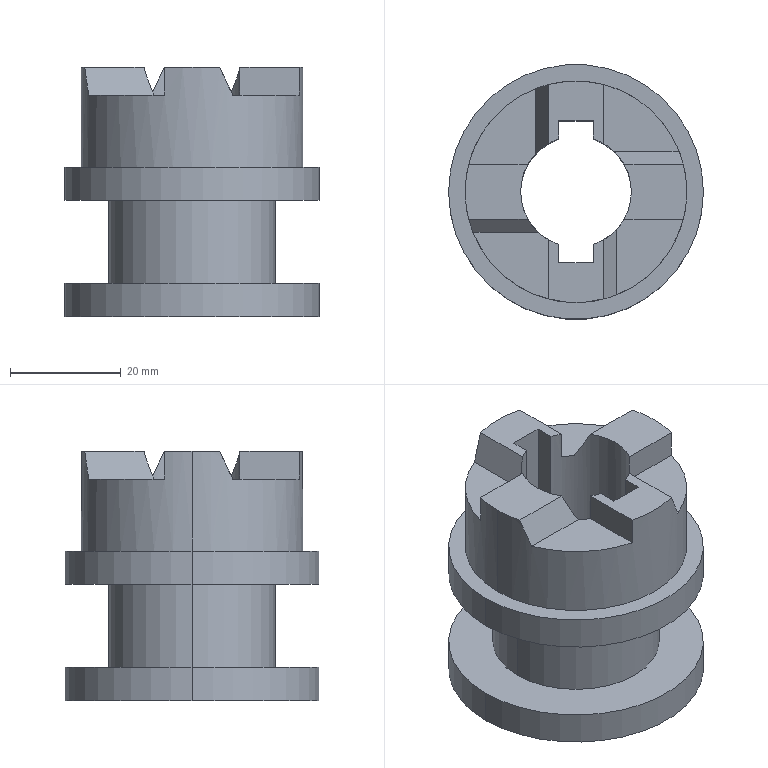Part | NX | features BREP 1, DATUM_CSYS 1, EXTRACT_DATUM_PLANE 1, SKETCH 1 | 1 solid | 37 faces | box 46 x 46 x 45 mm | volume 34964 mm3 | plane 26 | cylinder 11 | commonest cylinder face diameters 46 x4 20 x3 30 x2 40 x2
STEP:
#1=CARTESIAN_POINT('',(3.1,-12.8,45.));
#2=VERTEX_POINT('',#1);
#3=CARTESIAN_POINT('',(3.1,-12.8,0.));
#4=VERTEX_POINT('',#3);
#5=CARTESIAN_POINT('',(3.1,-12.8,45.));
#6=DIRECTION('',(0.,0.,-1.));
#7=VECTOR('',#6,1000.);
#8=LINE('',#5,#7);
#9=EDGE_CURVE('',#2,#4,#8,.T.);
#10=ORIENTED_EDGE('',*,*,#9,.T.);
#11=CARTESIAN_POINT('',(-3.1,-12.8,0.));
#12=VERTEX_POINT('',#11);
#13=CARTESIAN_POINT('',(3.1,-12.8,0.));
#14=DIRECTION('',(-1.,0.,0.));
#15=VECTOR('',#14,1000.);
#16=LINE('',#13,#15);
#17=EDGE_CURVE('',#4,#12,#16,.T.);
#18=ORIENTED_EDGE('',*,*,#17,.T.);
#19=CARTESIAN_POINT('',(-3.1,-12.8,45.));
#20=VERTEX_POINT('',#19);
#21=CARTESIAN_POINT('',(-3.1,-12.8,45.));
#22=DIRECTION('',(0.,0.,-1.));
#23=VECTOR('',#22,1000.);
#24=LINE('',#21,#23);
#25=EDGE_CURVE('',#20,#12,#24,.T.);
#26=ORIENTED_EDGE('',*,*,#25,.F.);
#27=CARTESIAN_POINT('',(3.1,-12.8,45.));
#28=DIRECTION('',(-1.,0.,0.));
#29=VECTOR('',#28,1000.);
#30=LINE('',#27,#29);
#31=EDGE_CURVE('',#2,#20,#30,.T.);
#32=ORIENTED_EDGE('',*,*,#31,.F.);
#33=EDGE_LOOP('',(#10,#18,#26,#32));
#34=FACE_BOUND('',#33,.T.);
#35=CARTESIAN_POINT('',(-3.1,-12.8,0.));
#36=DIRECTION('',(0.,-1.,0.));
#37=DIRECTION('',(0.,0.,1.));
#38=AXIS2_PLACEMENT_3D('',#35,#36,#37);
#39=PLANE('',#38);
#40=ADVANCED_FACE('',(#34),#39,.F.);
#41=CARTESIAN_POINT('',(-3.1,-9.507,45.));
#42=VERTEX_POINT('',#41);
#43=CARTESIAN_POINT('',(-3.1,-12.8,45.));
#44=DIRECTION('',(0.,1.,0.));
#45=VECTOR('',#44,1000.);
#46=LINE('',#43,#45);
#47=EDGE_CURVE('',#20,#42,#46,.T.);
#48=ORIENTED_EDGE('',*,*,#47,.T.);
#49=CARTESIAN_POINT('',(-5.,-8.66,45.));
#50=VERTEX_POINT('',#49);
#51=CARTESIAN_POINT('',(0.,0.,45.));
#52=DIRECTION('',(0.,0.,-1.));
#53=DIRECTION('',(-0.31,-0.9507,0.));
#54=AXIS2_PLACEMENT_3D('',#51,#52,#53);
#55=CIRCLE('',#54,10.);
#56=EDGE_CURVE('',#42,#50,#55,.T.);
#57=ORIENTED_EDGE('',*,*,#56,.T.);
#58=CARTESIAN_POINT('',(-5.,-19.365,45.));
#59=VERTEX_POINT('',#58);
#60=CARTESIAN_POINT('',(-5.,-8.66,45.));
#61=DIRECTION('',(0.,-1.,0.));
#62=VECTOR('',#61,1000.);
#63=LINE('',#60,#62);
#64=EDGE_CURVE('',#50,#59,#63,.T.);
#65=ORIENTED_EDGE('',*,*,#64,.T.);
#66=CARTESIAN_POINT('',(5.,-19.365,45.));
#67=VERTEX_POINT('',#66);
#68=CARTESIAN_POINT('',(0.,0.,45.));
#69=DIRECTION('',(0.,0.,1.));
#70=DIRECTION('',(-0.25,-0.9682,0.));
#71=AXIS2_PLACEMENT_3D('',#68,#69,#70);
#72=CIRCLE('',#71,20.);
#73=EDGE_CURVE('',#59,#67,#72,.T.);
#74=ORIENTED_EDGE('',*,*,#73,.T.);
#75=CARTESIAN_POINT('',(5.,-8.66,45.));
#76=VERTEX_POINT('',#75);
#77=CARTESIAN_POINT('',(5.,-8.66,45.));
#78=DIRECTION('',(0.,-1.,0.));
#79=VECTOR('',#78,1000.);
#80=LINE('',#77,#79);
#81=EDGE_CURVE('',#76,#67,#80,.T.);
#82=ORIENTED_EDGE('',*,*,#81,.F.);
#83=CARTESIAN_POINT('',(3.1,-9.507,45.));
#84=VERTEX_POINT('',#83);
#85=CARTESIAN_POINT('',(0.,0.,45.));
#86=DIRECTION('',(0.,0.,-1.));
#87=DIRECTION('',(0.5,-0.866,0.));
#88=AXIS2_PLACEMENT_3D('',#85,#86,#87);
#89=CIRCLE('',#88,10.);
#90=EDGE_CURVE('',#76,#84,#89,.T.);
#91=ORIENTED_EDGE('',*,*,#90,.T.);
#92=CARTESIAN_POINT('',(3.1,-9.507,45.));
#93=DIRECTION('',(0.,-1.,0.));
#94=VECTOR('',#93,1000.);
#95=LINE('',#92,#94);
#96=EDGE_CURVE('',#84,#2,#95,.T.);
#97=ORIENTED_EDGE('',*,*,#96,.T.);
#98=ORIENTED_EDGE('',*,*,#31,.T.);
#99=EDGE_LOOP('',(#48,#57,#65,#74,#82,#91,#97,#98));
#100=FACE_BOUND('',#99,.T.);
#101=CARTESIAN_POINT('',(-5.,28.,45.));
#102=DIRECTION('',(0.,0.,-1.));
#103=DIRECTION('',(1.,0.,0.));
#104=AXIS2_PLACEMENT_3D('',#101,#102,#103);
#105=PLANE('',#104);
#106=ADVANCED_FACE('',(#100),#105,.F.);
#107=CARTESIAN_POINT('',(3.1,-9.507,0.));
#108=VERTEX_POINT('',#107);
#109=CARTESIAN_POINT('',(3.1,-9.507,0.));
#110=DIRECTION('',(0.,-1.,0.));
#111=VECTOR('',#110,1000.);
#112=LINE('',#109,#111);
#113=EDGE_CURVE('',#108,#4,#112,.T.);
#114=ORIENTED_EDGE('',*,*,#113,.T.);
#115=ORIENTED_EDGE('',*,*,#9,.F.);
#116=ORIENTED_EDGE('',*,*,#96,.F.);
#117=CARTESIAN_POINT('',(3.1,-9.507,0.));
#118=DIRECTION('',(0.,0.,1.));
#119=VECTOR('',#118,1000.);
#120=LINE('',#117,#119);
#121=EDGE_CURVE('',#108,#84,#120,.T.);
#122=ORIENTED_EDGE('',*,*,#121,.F.);
#123=EDGE_LOOP('',(#114,#115,#116,#122));
#124=FACE_BOUND('',#123,.T.);
#125=CARTESIAN_POINT('',(3.1,-12.8,0.));
#126=DIRECTION('',(1.,0.,0.));
#127=DIRECTION('',(0.,-1.,0.));
#128=AXIS2_PLACEMENT_3D('',#125,#126,#127);
#129=PLANE('',#128);
#130=ADVANCED_FACE('',(#124),#129,.F.);
#131=ORIENTED_EDGE('',*,*,#90,.F.);
#132=CARTESIAN_POINT('',(7.332,-6.801,40.));
#133=VERTEX_POINT('',#132);
#134=CARTESIAN_POINT('',(0.,0.,55.723));
#135=DIRECTION('',(-0.9063,0.,-0.4226));
#136=DIRECTION('',(0.4226,0.,-0.9063));
#137=AXIS2_PLACEMENT_3D('',#134,#135,#136);
#138=ELLIPSE('',#137,23.662,10.);
#139=EDGE_CURVE('',#133,#76,#138,.T.);
#140=ORIENTED_EDGE('',*,*,#139,.F.);
#141=CARTESIAN_POINT('',(8.66,-5.,40.));
#142=VERTEX_POINT('',#141);
#143=CARTESIAN_POINT('',(0.,0.,40.));
#144=DIRECTION('',(0.,0.,-1.));
#145=DIRECTION('',(0.866,-0.5,0.));
#146=AXIS2_PLACEMENT_3D('',#143,#144,#145);
#147=CIRCLE('',#146,10.);
#148=EDGE_CURVE('',#142,#133,#147,.T.);
#149=ORIENTED_EDGE('',*,*,#148,.F.);
#150=CARTESIAN_POINT('',(8.66,-5.,45.));
#151=VERTEX_POINT('',#150);
#152=CARTESIAN_POINT('',(8.66,-5.,40.));
#153=DIRECTION('',(0.000000002,0.,1.));
#154=VECTOR('',#153,1000.);
#155=LINE('',#152,#154);
#156=EDGE_CURVE('',#142,#151,#155,.T.);
#157=ORIENTED_EDGE('',*,*,#156,.T.);
#158=CARTESIAN_POINT('',(10.,0.,45.));
#159=VERTEX_POINT('',#158);
#160=CARTESIAN_POINT('',(0.,0.,45.));
#161=DIRECTION('',(0.,0.,-1.));
#162=DIRECTION('',(1.,0.,0.));
#163=AXIS2_PLACEMENT_3D('',#160,#161,#162);
#164=CIRCLE('',#163,10.);
#165=EDGE_CURVE('',#159,#151,#164,.T.);
#166=ORIENTED_EDGE('',*,*,#165,.F.);
#167=CARTESIAN_POINT('',(8.66,5.,45.));
#168=VERTEX_POINT('',#167);
#169=CARTESIAN_POINT('',(0.,0.,45.));
#170=DIRECTION('',(0.,0.,-1.));
#171=DIRECTION('',(0.866,0.5,0.));
#172=AXIS2_PLACEMENT_3D('',#169,#170,#171);
#173=CIRCLE('',#172,10.);
#174=EDGE_CURVE('',#168,#159,#173,.T.);
#175=ORIENTED_EDGE('',*,*,#174,.F.);
#176=CARTESIAN_POINT('',(6.801,7.332,40.));
#177=VERTEX_POINT('',#176);
#178=CARTESIAN_POINT('',(0.,0.,55.723));
#179=DIRECTION('',(0.,-0.9063,-0.4226));
#180=DIRECTION('',(0.,0.4226,-0.9063));
#181=AXIS2_PLACEMENT_3D('',#178,#179,#180);
#182=ELLIPSE('',#181,23.662,10.);
#183=EDGE_CURVE('',#177,#168,#182,.T.);
#184=ORIENTED_EDGE('',*,*,#183,.F.);
#185=CARTESIAN_POINT('',(5.,8.66,40.));
#186=VERTEX_POINT('',#185);
#187=CARTESIAN_POINT('',(0.,0.,40.));
#188=DIRECTION('',(0.,0.,-1.));
#189=DIRECTION('',(0.5,0.866,0.));
#190=AXIS2_PLACEMENT_3D('',#187,#188,#189);
#191=CIRCLE('',#190,10.);
#192=EDGE_CURVE('',#186,#177,#191,.T.);
#193=ORIENTED_EDGE('',*,*,#192,.F.);
#194=CARTESIAN_POINT('',(5.,8.66,45.));
#195=VERTEX_POINT('',#194);
#196=CARTESIAN_POINT('',(5.,8.66,40.));
#197=DIRECTION('',(0.,0.000000001,1.));
#198=VECTOR('',#197,1000.);
#199=LINE('',#196,#198);
#200=EDGE_CURVE('',#186,#195,#199,.T.);
#201=ORIENTED_EDGE('',*,*,#200,.T.);
#202=CARTESIAN_POINT('',(3.1,9.507,45.));
#203=VERTEX_POINT('',#202);
#204=CARTESIAN_POINT('',(0.,0.,45.));
#205=DIRECTION('',(0.,0.,-1.));
#206=DIRECTION('',(0.31,0.9507,0.));
#207=AXIS2_PLACEMENT_3D('',#204,#205,#206);
#208=CIRCLE('',#207,10.);
#209=EDGE_CURVE('',#203,#195,#208,.T.);
#210=ORIENTED_EDGE('',*,*,#209,.F.);
#211=CARTESIAN_POINT('',(3.1,9.507,0.));
#212=VERTEX_POINT('',#211);
#213=CARTESIAN_POINT('',(3.1,9.507,45.));
#214=DIRECTION('',(0.,0.,-1.));
#215=VECTOR('',#214,1000.);
#216=LINE('',#213,#215);
#217=EDGE_CURVE('',#203,#212,#216,.T.);
#218=ORIENTED_EDGE('',*,*,#217,.T.);
#219=CARTESIAN_POINT('',(0.,0.,0.));
#220=DIRECTION('',(0.,0.,1.));
#221=DIRECTION('',(0.31,-0.9507,0.));
#222=AXIS2_PLACEMENT_3D('',#219,#220,#221);
#223=CIRCLE('',#222,10.);
#224=EDGE_CURVE('',#108,#212,#223,.T.);
#225=ORIENTED_EDGE('',*,*,#224,.F.);
#226=ORIENTED_EDGE('',*,*,#121,.T.);
#227=EDGE_LOOP('',(#131,#140,#149,#157,#166,#175,#184,#193,#201,#210,#218,#225,#226));
#228=FACE_BOUND('',#227,.T.);
#229=CARTESIAN_POINT('',(0.,0.,40.));
#230=DIRECTION('',(0.,0.,-1.));
#231=DIRECTION('',(1.,0.,0.));
#232=AXIS2_PLACEMENT_3D('',#229,#230,#231);
#233=CYLINDRICAL_SURFACE('',#232,10.);
#234=ADVANCED_FACE('',(#228),#233,.F.);
#235=CARTESIAN_POINT('',(23.,0.,0.));
#236=VERTEX_POINT('',#235);
#237=CARTESIAN_POINT('',(-23.,0.,0.));
#238=VERTEX_POINT('',#237);
#239=CARTESIAN_POINT('',(0.,0.,0.));
#240=DIRECTION('',(0.,0.,-1.));
#241=DIRECTION('',(1.,0.,0.));
#242=AXIS2_PLACEMENT_3D('',#239,#240,#241);
#243=CIRCLE('',#242,23.);
#244=EDGE_CURVE('',#236,#238,#243,.T.);
#245=ORIENTED_EDGE('',*,*,#244,.T.);
#246=CARTESIAN_POINT('',(0.,0.,0.));
#247=DIRECTION('',(0.,0.,-1.));
#248=DIRECTION('',(-1.,0.,0.));
#249=AXIS2_PLACEMENT_3D('',#246,#247,#248);
#250=CIRCLE('',#249,23.);
#251=EDGE_CURVE('',#238,#236,#250,.T.);
#252=ORIENTED_EDGE('',*,*,#251,.T.);
#253=EDGE_LOOP('',(#245,#252));
#254=FACE_BOUND('',#253,.T.);
#255=CARTESIAN_POINT('',(-10.,0.,0.));
#256=VERTEX_POINT('',#255);
#257=CARTESIAN_POINT('',(-3.1,-9.507,0.));
#258=VERTEX_POINT('',#257);
#259=CARTESIAN_POINT('',(0.,0.,0.));
#260=DIRECTION('',(0.,0.,1.));
#261=DIRECTION('',(-1.,0.,0.));
#262=AXIS2_PLACEMENT_3D('',#259,#260,#261);
#263=CIRCLE('',#262,10.);
#264=EDGE_CURVE('',#256,#258,#263,.T.);
#265=ORIENTED_EDGE('',*,*,#264,.T.);
#266=CARTESIAN_POINT('',(-3.1,-12.8,0.));
#267=DIRECTION('',(0.,1.,0.));
#268=VECTOR('',#267,1000.);
#269=LINE('',#266,#268);
#270=EDGE_CURVE('',#12,#258,#269,.T.);
#271=ORIENTED_EDGE('',*,*,#270,.F.);
#272=ORIENTED_EDGE('',*,*,#17,.F.);
#273=ORIENTED_EDGE('',*,*,#113,.F.);
#274=ORIENTED_EDGE('',*,*,#224,.T.);
#275=CARTESIAN_POINT('',(3.1,12.8,0.));
#276=VERTEX_POINT('',#275);
#277=CARTESIAN_POINT('',(3.1,12.8,0.));
#278=DIRECTION('',(0.,-1.,0.));
#279=VECTOR('',#278,1000.);
#280=LINE('',#277,#279);
#281=EDGE_CURVE('',#276,#212,#280,.T.);
#282=ORIENTED_EDGE('',*,*,#281,.F.);
#283=CARTESIAN_POINT('',(-3.1,12.8,0.));
#284=VERTEX_POINT('',#283);
#285=CARTESIAN_POINT('',(-3.1,12.8,0.));
#286=DIRECTION('',(1.,0.,0.));
#287=VECTOR('',#286,1000.);
#288=LINE('',#285,#287);
#289=EDGE_CURVE('',#284,#276,#288,.T.);
#290=ORIENTED_EDGE('',*,*,#289,.F.);
#291=CARTESIAN_POINT('',(-3.1,9.507,0.));
#292=VERTEX_POINT('',#291);
#293=CARTESIAN_POINT('',(-3.1,9.507,0.));
#294=DIRECTION('',(0.,1.,0.));
#295=VECTOR('',#294,1000.);
#296=LINE('',#293,#295);
#297=EDGE_CURVE('',#292,#284,#296,.T.);
#298=ORIENTED_EDGE('',*,*,#297,.F.);
#299=CARTESIAN_POINT('',(0.,0.,0.));
#300=DIRECTION('',(0.,0.,1.));
#301=DIRECTION('',(-0.31,0.9507,0.));
#302=AXIS2_PLACEMENT_3D('',#299,#300,#301);
#303=CIRCLE('',#302,10.);
#304=EDGE_CURVE('',#292,#256,#303,.T.);
#305=ORIENTED_EDGE('',*,*,#304,.T.);
#306=EDGE_LOOP('',(#265,#271,#272,#273,#274,#282,#290,#298,#305));
#307=FACE_BOUND('',#306,.T.);
#308=CARTESIAN_POINT('',(0.,0.,0.));
#309=DIRECTION('',(0.,0.,1.));
#310=DIRECTION('',(-1.,0.,0.));
#311=AXIS2_PLACEMENT_3D('',#308,#309,#310);
#312=PLANE('',#311);
#313=ADVANCED_FACE('',(#254,#307),#312,.F.);
#314=CARTESIAN_POINT('',(23.,0.,6.));
#315=VERTEX_POINT('',#314);
#316=CARTESIAN_POINT('',(23.,0.,0.));
#317=DIRECTION('',(0.,0.,1.));
#318=VECTOR('',#317,1000.);
#319=LINE('',#316,#318);
#320=EDGE_CURVE('',#236,#315,#319,.T.);
#321=ORIENTED_EDGE('',*,*,#320,.F.);
#322=ORIENTED_EDGE('',*,*,#251,.F.);
#323=CARTESIAN_POINT('',(-23.,0.,6.));
#324=VERTEX_POINT('',#323);
#325=CARTESIAN_POINT('',(-23.,0.,0.));
#326=DIRECTION('',(0.,0.,1.));
#327=VECTOR('',#326,1000.);
#328=LINE('',#325,#327);
#329=EDGE_CURVE('',#238,#324,#328,.T.);
#330=ORIENTED_EDGE('',*,*,#329,.T.);
#331=CARTESIAN_POINT('',(0.,0.,6.));
#332=DIRECTION('',(0.,0.,1.));
#333=DIRECTION('',(1.,0.,0.));
#334=AXIS2_PLACEMENT_3D('',#331,#332,#333);
#335=CIRCLE('',#334,23.);
#336=EDGE_CURVE('',#315,#324,#335,.T.);
#337=ORIENTED_EDGE('',*,*,#336,.F.);
#338=EDGE_LOOP('',(#321,#322,#330,#337));
#339=FACE_BOUND('',#338,.T.);
#340=CARTESIAN_POINT('',(0.,0.,0.));
#341=DIRECTION('',(0.,0.,-1.));
#342=DIRECTION('',(1.,0.,0.));
#343=AXIS2_PLACEMENT_3D('',#340,#341,#342);
#344=CYLINDRICAL_SURFACE('',#343,23.);
#345=ADVANCED_FACE('',(#339),#344,.T.);
#346=CARTESIAN_POINT('',(0.,0.,6.));
#347=DIRECTION('',(0.,0.,1.));
#348=DIRECTION('',(-1.,0.,0.));
#349=AXIS2_PLACEMENT_3D('',#346,#347,#348);
#350=CIRCLE('',#349,23.);
#351=EDGE_CURVE('',#324,#315,#350,.T.);
#352=ORIENTED_EDGE('',*,*,#351,.T.);
#353=ORIENTED_EDGE('',*,*,#336,.T.);
#354=EDGE_LOOP('',(#352,#353));
#355=FACE_BOUND('',#354,.T.);
#356=CARTESIAN_POINT('',(15.,0.,6.));
#357=VERTEX_POINT('',#356);
#358=CARTESIAN_POINT('',(-15.,0.,6.));
#359=VERTEX_POINT('',#358);
#360=CARTESIAN_POINT('',(0.,0.,6.));
#361=DIRECTION('',(0.,0.,-1.));
#362=DIRECTION('',(1.,0.,0.));
#363=AXIS2_PLACEMENT_3D('',#360,#361,#362);
#364=CIRCLE('',#363,15.);
#365=EDGE_CURVE('',#357,#359,#364,.T.);
#366=ORIENTED_EDGE('',*,*,#365,.T.);
#367=CARTESIAN_POINT('',(0.,0.,6.));
#368=DIRECTION('',(0.,0.,-1.));
#369=DIRECTION('',(-1.,0.,0.));
#370=AXIS2_PLACEMENT_3D('',#367,#368,#369);
#371=CIRCLE('',#370,15.);
#372=EDGE_CURVE('',#359,#357,#371,.T.);
#373=ORIENTED_EDGE('',*,*,#372,.T.);
#374=EDGE_LOOP('',(#366,#373));
#375=FACE_BOUND('',#374,.T.);
#376=CARTESIAN_POINT('',(15.,0.,6.));
#377=DIRECTION('',(0.,0.,-1.));
#378=DIRECTION('',(1.,0.,0.));
#379=AXIS2_PLACEMENT_3D('',#376,#377,#378);
#380=PLANE('',#379);
#381=ADVANCED_FACE('',(#355,#375),#380,.F.);
#382=ORIENTED_EDGE('',*,*,#351,.F.);
#383=ORIENTED_EDGE('',*,*,#329,.F.);
#384=ORIENTED_EDGE('',*,*,#244,.F.);
#385=ORIENTED_EDGE('',*,*,#320,.T.);
#386=EDGE_LOOP('',(#382,#383,#384,#385));
#387=FACE_BOUND('',#386,.T.);
#388=CARTESIAN_POINT('',(0.,0.,0.));
#389=DIRECTION('',(0.,0.,-1.));
#390=DIRECTION('',(1.,0.,0.));
#391=AXIS2_PLACEMENT_3D('',#388,#389,#390);
#392=CYLINDRICAL_SURFACE('',#391,23.);
#393=ADVANCED_FACE('',(#387),#392,.T.);
#394=CARTESIAN_POINT('',(-15.,0.,21.));
#395=VERTEX_POINT('',#394);
#396=CARTESIAN_POINT('',(-15.,0.,21.));
#397=DIRECTION('',(0.,0.,-1.));
#398=VECTOR('',#397,1000.);
#399=LINE('',#396,#398);
#400=EDGE_CURVE('',#359,#395,#399,.F.);
#401=ORIENTED_EDGE('',*,*,#400,.T.);
#402=CARTESIAN_POINT('',(15.,0.,21.));
#403=VERTEX_POINT('',#402);
#404=CARTESIAN_POINT('',(0.,0.,21.));
#405=DIRECTION('',(0.,0.,1.));
#406=DIRECTION('',(1.,0.,0.));
#407=AXIS2_PLACEMENT_3D('',#404,#405,#406);
#408=CIRCLE('',#407,15.);
#409=EDGE_CURVE('',#403,#395,#408,.T.);
#410=ORIENTED_EDGE('',*,*,#409,.F.);
#411=CARTESIAN_POINT('',(15.,0.,21.));
#412=DIRECTION('',(0.,0.,-1.));
#413=VECTOR('',#412,1000.);
#414=LINE('',#411,#413);
#415=EDGE_CURVE('',#357,#403,#414,.F.);
#416=ORIENTED_EDGE('',*,*,#415,.F.);
#417=ORIENTED_EDGE('',*,*,#372,.F.);
#418=EDGE_LOOP('',(#401,#410,#416,#417));
#419=FACE_BOUND('',#418,.T.);
#420=CARTESIAN_POINT('',(0.,0.,0.));
#421=DIRECTION('',(0.,0.,1.));
#422=DIRECTION('',(-1.,0.,0.));
#423=AXIS2_PLACEMENT_3D('',#420,#421,#422);
#424=CYLINDRICAL_SURFACE('',#423,15.);
#425=ADVANCED_FACE('',(#419),#424,.T.);
#426=ORIENTED_EDGE('',*,*,#365,.F.);
#427=ORIENTED_EDGE('',*,*,#415,.T.);
#428=CARTESIAN_POINT('',(0.,0.,21.));
#429=DIRECTION('',(0.,0.,1.));
#430=DIRECTION('',(-1.,0.,0.));
#431=AXIS2_PLACEMENT_3D('',#428,#429,#430);
#432=CIRCLE('',#431,15.);
#433=EDGE_CURVE('',#395,#403,#432,.T.);
#434=ORIENTED_EDGE('',*,*,#433,.F.);
#435=ORIENTED_EDGE('',*,*,#400,.F.);
#436=EDGE_LOOP('',(#426,#427,#434,#435));
#437=FACE_BOUND('',#436,.T.);
#438=CARTESIAN_POINT('',(0.,0.,0.));
#439=DIRECTION('',(0.,0.,1.));
#440=DIRECTION('',(-1.,0.,0.));
#441=AXIS2_PLACEMENT_3D('',#438,#439,#440);
#442=CYLINDRICAL_SURFACE('',#441,15.);
#443=ADVANCED_FACE('',(#437),#442,.T.);
#444=CARTESIAN_POINT('',(23.,0.,21.));
#445=VERTEX_POINT('',#444);
#446=CARTESIAN_POINT('',(-23.,0.,21.));
#447=VERTEX_POINT('',#446);
#448=CARTESIAN_POINT('',(0.,0.,21.));
#449=DIRECTION('',(0.,0.,-1.));
#450=DIRECTION('',(1.,0.,0.));
#451=AXIS2_PLACEMENT_3D('',#448,#449,#450);
#452=CIRCLE('',#451,23.);
#453=EDGE_CURVE('',#445,#447,#452,.T.);
#454=ORIENTED_EDGE('',*,*,#453,.T.);
#455=CARTESIAN_POINT('',(0.,0.,21.));
#456=DIRECTION('',(0.,0.,-1.));
#457=DIRECTION('',(-1.,0.,0.));
#458=AXIS2_PLACEMENT_3D('',#455,#456,#457);
#459=CIRCLE('',#458,23.);
#460=EDGE_CURVE('',#447,#445,#459,.T.);
#461=ORIENTED_EDGE('',*,*,#460,.T.);
#462=EDGE_LOOP('',(#454,#461));
#463=FACE_BOUND('',#462,.T.);
#464=ORIENTED_EDGE('',*,*,#433,.T.);
#465=ORIENTED_EDGE('',*,*,#409,.T.);
#466=EDGE_LOOP('',(#464,#465));
#467=FACE_BOUND('',#466,.T.);
#468=CARTESIAN_POINT('',(15.,0.,21.));
#469=DIRECTION('',(0.,0.,1.));
#470=DIRECTION('',(-1.,0.,0.));
#471=AXIS2_PLACEMENT_3D('',#468,#469,#470);
#472=PLANE('',#471);
#473=ADVANCED_FACE('',(#463,#467),#472,.F.);
#474=CARTESIAN_POINT('',(23.,0.,27.));
#475=VERTEX_POINT('',#474);
#476=CARTESIAN_POINT('',(23.,0.,21.));
#477=DIRECTION('',(0.,0.,1.));
#478=VECTOR('',#477,1000.);
#479=LINE('',#476,#478);
#480=EDGE_CURVE('',#445,#475,#479,.T.);
#481=ORIENTED_EDGE('',*,*,#480,.F.);
#482=ORIENTED_EDGE('',*,*,#460,.F.);
#483=CARTESIAN_POINT('',(-23.,0.,27.));
#484=VERTEX_POINT('',#483);
#485=CARTESIAN_POINT('',(-23.,0.,21.));
#486=DIRECTION('',(0.,0.,1.));
#487=VECTOR('',#486,1000.);
#488=LINE('',#485,#487);
#489=EDGE_CURVE('',#447,#484,#488,.T.);
#490=ORIENTED_EDGE('',*,*,#489,.T.);
#491=CARTESIAN_POINT('',(0.,0.,27.));
#492=DIRECTION('',(0.,0.,1.));
#493=DIRECTION('',(1.,0.,0.));
#494=AXIS2_PLACEMENT_3D('',#491,#492,#493);
#495=CIRCLE('',#494,23.);
#496=EDGE_CURVE('',#475,#484,#495,.T.);
#497=ORIENTED_EDGE('',*,*,#496,.F.);
#498=EDGE_LOOP('',(#481,#482,#490,#497));
#499=FACE_BOUND('',#498,.T.);
#500=CARTESIAN_POINT('',(0.,0.,0.));
#501=DIRECTION('',(0.,0.,-1.));
#502=DIRECTION('',(1.,0.,0.));
#503=AXIS2_PLACEMENT_3D('',#500,#501,#502);
#504=CYLINDRICAL_SURFACE('',#503,23.);
#505=ADVANCED_FACE('',(#499),#504,.T.);
#506=CARTESIAN_POINT('',(0.,0.,27.));
#507=DIRECTION('',(0.,0.,1.));
#508=DIRECTION('',(-1.,0.,0.));
#509=AXIS2_PLACEMENT_3D('',#506,#507,#508);
#510=CIRCLE('',#509,23.);
#511=EDGE_CURVE('',#484,#475,#510,.T.);
#512=ORIENTED_EDGE('',*,*,#511,.T.);
#513=ORIENTED_EDGE('',*,*,#496,.T.);
#514=EDGE_LOOP('',(#512,#513));
#515=FACE_BOUND('',#514,.T.);
#516=CARTESIAN_POINT('',(20.,0.,27.));
#517=VERTEX_POINT('',#516);
#518=CARTESIAN_POINT('',(-20.,0.,27.));
#519=VERTEX_POINT('',#518);
#520=CARTESIAN_POINT('',(0.,0.,27.));
#521=DIRECTION('',(0.,0.,-1.));
#522=DIRECTION('',(1.,0.,0.));
#523=AXIS2_PLACEMENT_3D('',#520,#521,#522);
#524=CIRCLE('',#523,20.);
#525=EDGE_CURVE('',#517,#519,#524,.T.);
#526=ORIENTED_EDGE('',*,*,#525,.T.);
#527=CARTESIAN_POINT('',(0.,0.,27.));
#528=DIRECTION('',(0.,0.,-1.));
#529=DIRECTION('',(-1.,0.,0.));
#530=AXIS2_PLACEMENT_3D('',#527,#528,#529);
#531=CIRCLE('',#530,20.);
#532=EDGE_CURVE('',#519,#517,#531,.T.);
#533=ORIENTED_EDGE('',*,*,#532,.T.);
#534=EDGE_LOOP('',(#526,#533));
#535=FACE_BOUND('',#534,.T.);
#536=CARTESIAN_POINT('',(20.,0.,27.));
#537=DIRECTION('',(0.,0.,-1.));
#538=DIRECTION('',(1.,0.,0.));
#539=AXIS2_PLACEMENT_3D('',#536,#537,#538);
#540=PLANE('',#539);
#541=ADVANCED_FACE('',(#515,#535),#540,.F.);
#542=ORIENTED_EDGE('',*,*,#511,.F.);
#543=ORIENTED_EDGE('',*,*,#489,.F.);
#544=ORIENTED_EDGE('',*,*,#453,.F.);
#545=ORIENTED_EDGE('',*,*,#480,.T.);
#546=EDGE_LOOP('',(#542,#543,#544,#545));
#547=FACE_BOUND('',#546,.T.);
#548=CARTESIAN_POINT('',(0.,0.,0.));
#549=DIRECTION('',(0.,0.,-1.));
#550=DIRECTION('',(1.,0.,0.));
#551=AXIS2_PLACEMENT_3D('',#548,#549,#550);
#552=CYLINDRICAL_SURFACE('',#551,23.);
#553=ADVANCED_FACE('',(#547),#552,.T.);
#554=CARTESIAN_POINT('',(20.,0.,45.));
#555=VERTEX_POINT('',#554);
#556=CARTESIAN_POINT('',(20.,0.,27.));
#557=DIRECTION('',(0.,0.,1.));
#558=VECTOR('',#557,1000.);
#559=LINE('',#556,#558);
#560=EDGE_CURVE('',#517,#555,#559,.T.);
#561=ORIENTED_EDGE('',*,*,#560,.F.);
#562=ORIENTED_EDGE('',*,*,#532,.F.);
#563=CARTESIAN_POINT('',(-20.,0.,45.));
#564=VERTEX_POINT('',#563);
#565=CARTESIAN_POINT('',(-20.,0.,27.));
#566=DIRECTION('',(0.,0.,1.));
#567=VECTOR('',#566,1000.);
#568=LINE('',#565,#567);
#569=EDGE_CURVE('',#519,#564,#568,.T.);
#570=ORIENTED_EDGE('',*,*,#569,.T.);
#571=CARTESIAN_POINT('',(-19.365,5.,45.));
#572=VERTEX_POINT('',#571);
#573=CARTESIAN_POINT('',(0.,0.,45.));
#574=DIRECTION('',(0.,0.,1.));
#575=DIRECTION('',(-0.9682,0.25,0.));
#576=AXIS2_PLACEMENT_3D('',#573,#574,#575);
#577=CIRCLE('',#576,20.);
#578=EDGE_CURVE('',#572,#564,#577,.T.);
#579=ORIENTED_EDGE('',*,*,#578,.F.);
#580=CARTESIAN_POINT('',(-19.365,5.,40.));
#581=VERTEX_POINT('',#580);
#582=CARTESIAN_POINT('',(-19.365,5.,45.));
#583=DIRECTION('',(0.,0.,-1.));
#584=VECTOR('',#583,1000.);
#585=LINE('',#582,#584);
#586=EDGE_CURVE('',#572,#581,#585,.T.);
#587=ORIENTED_EDGE('',*,*,#586,.T.);
#588=CARTESIAN_POINT('',(-7.332,18.608,40.));
#589=VERTEX_POINT('',#588);
#590=CARTESIAN_POINT('',(0.,0.,40.));
#591=DIRECTION('',(0.,0.,1.));
#592=DIRECTION('',(-0.3666,0.9304,0.));
#593=AXIS2_PLACEMENT_3D('',#590,#591,#592);
#594=CIRCLE('',#593,20.);
#595=EDGE_CURVE('',#589,#581,#594,.T.);
#596=ORIENTED_EDGE('',*,*,#595,.F.);
#597=CARTESIAN_POINT('',(-5.,19.365,45.));
#598=VERTEX_POINT('',#597);
#599=CARTESIAN_POINT('',(0.,0.,55.723));
#600=DIRECTION('',(0.9063,0.,-0.4226));
#601=DIRECTION('',(-0.4226,0.,-0.9063));
#602=AXIS2_PLACEMENT_3D('',#599,#600,#601);
#603=ELLIPSE('',#602,47.324,20.);
#604=EDGE_CURVE('',#598,#589,#603,.F.);
#605=ORIENTED_EDGE('',*,*,#604,.F.);
#606=CARTESIAN_POINT('',(5.,19.365,45.));
#607=VERTEX_POINT('',#606);
#608=CARTESIAN_POINT('',(0.,0.,45.));
#609=DIRECTION('',(0.,0.,1.));
#610=DIRECTION('',(0.25,0.9682,0.));
#611=AXIS2_PLACEMENT_3D('',#608,#609,#610);
#612=CIRCLE('',#611,20.);
#613=EDGE_CURVE('',#607,#598,#612,.T.);
#614=ORIENTED_EDGE('',*,*,#613,.F.);
#615=CARTESIAN_POINT('',(5.,19.365,40.));
#616=VERTEX_POINT('',#615);
#617=CARTESIAN_POINT('',(5.,19.365,45.));
#618=DIRECTION('',(0.,0.,-1.));
#619=VECTOR('',#618,1000.);
#620=LINE('',#617,#619);
#621=EDGE_CURVE('',#607,#616,#620,.T.);
#622=ORIENTED_EDGE('',*,*,#621,.T.);
#623=CARTESIAN_POINT('',(18.608,7.332,40.));
#624=VERTEX_POINT('',#623);
#625=CARTESIAN_POINT('',(0.,0.,40.));
#626=DIRECTION('',(0.,0.,1.));
#627=DIRECTION('',(0.9304,0.3666,0.));
#628=AXIS2_PLACEMENT_3D('',#625,#626,#627);
#629=CIRCLE('',#628,20.);
#630=EDGE_CURVE('',#624,#616,#629,.T.);
#631=ORIENTED_EDGE('',*,*,#630,.F.);
#632=CARTESIAN_POINT('',(19.365,5.,45.));
#633=VERTEX_POINT('',#632);
#634=CARTESIAN_POINT('',(0.,0.,55.723));
#635=DIRECTION('',(0.,-0.9063,-0.4226));
#636=DIRECTION('',(0.,0.4226,-0.9063));
#637=AXIS2_PLACEMENT_3D('',#634,#635,#636);
#638=ELLIPSE('',#637,47.324,20.);
#639=EDGE_CURVE('',#633,#624,#638,.F.);
#640=ORIENTED_EDGE('',*,*,#639,.F.);
#641=CARTESIAN_POINT('',(0.,0.,45.));
#642=DIRECTION('',(0.,0.,1.));
#643=DIRECTION('',(1.,0.,0.));
#644=AXIS2_PLACEMENT_3D('',#641,#642,#643);
#645=CIRCLE('',#644,20.);
#646=EDGE_CURVE('',#555,#633,#645,.T.);
#647=ORIENTED_EDGE('',*,*,#646,.F.);
#648=EDGE_LOOP('',(#561,#562,#570,#579,#587,#596,#605,#614,#622,#631,#640,#647));
#649=FACE_BOUND('',#648,.T.);
#650=CARTESIAN_POINT('',(0.,0.,40.));
#651=DIRECTION('',(0.,0.,-1.));
#652=DIRECTION('',(1.,0.,0.));
#653=AXIS2_PLACEMENT_3D('',#650,#651,#652);
#654=CYLINDRICAL_SURFACE('',#653,20.);
#655=ADVANCED_FACE('',(#649),#654,.T.);
#656=ORIENTED_EDGE('',*,*,#165,.T.);
#657=CARTESIAN_POINT('',(19.365,-5.,45.));
#658=VERTEX_POINT('',#657);
#659=CARTESIAN_POINT('',(8.66,-5.,45.));
#660=DIRECTION('',(1.,0.,0.));
#661=VECTOR('',#660,1000.);
#662=LINE('',#659,#661);
#663=EDGE_CURVE('',#151,#658,#662,.T.);
#664=ORIENTED_EDGE('',*,*,#663,.T.);
#665=CARTESIAN_POINT('',(0.,0.,45.));
#666=DIRECTION('',(0.,0.,1.));
#667=DIRECTION('',(0.9682,-0.25,0.));
#668=AXIS2_PLACEMENT_3D('',#665,#666,#667);
#669=CIRCLE('',#668,20.);
#670=EDGE_CURVE('',#658,#555,#669,.T.);
#671=ORIENTED_EDGE('',*,*,#670,.T.);
#672=ORIENTED_EDGE('',*,*,#646,.T.);
#673=CARTESIAN_POINT('',(8.66,5.,45.));
#674=DIRECTION('',(1.,0.,0.));
#675=VECTOR('',#674,1000.);
#676=LINE('',#673,#675);
#677=EDGE_CURVE('',#168,#633,#676,.T.);
#678=ORIENTED_EDGE('',*,*,#677,.F.);
#679=ORIENTED_EDGE('',*,*,#174,.T.);
#680=EDGE_LOOP('',(#656,#664,#671,#672,#678,#679));
#681=FACE_BOUND('',#680,.T.);
#682=CARTESIAN_POINT('',(-5.,28.,45.));
#683=DIRECTION('',(0.,0.,-1.));
#684=DIRECTION('',(1.,0.,0.));
#685=AXIS2_PLACEMENT_3D('',#682,#683,#684);
#686=PLANE('',#685);
#687=ADVANCED_FACE('',(#681),#686,.F.);
#688=ORIENTED_EDGE('',*,*,#677,.T.);
#689=ORIENTED_EDGE('',*,*,#639,.T.);
#690=CARTESIAN_POINT('',(6.801,7.332,40.));
#691=DIRECTION('',(1.,0.,0.));
#692=VECTOR('',#691,1000.);
#693=LINE('',#690,#692);
#694=EDGE_CURVE('',#177,#624,#693,.T.);
#695=ORIENTED_EDGE('',*,*,#694,.F.);
#696=ORIENTED_EDGE('',*,*,#183,.T.);
#697=EDGE_LOOP('',(#688,#689,#695,#696));
#698=FACE_BOUND('',#697,.T.);
#699=CARTESIAN_POINT('',(28.,5.,45.));
#700=DIRECTION('',(0.,-0.9063,-0.4226));
#701=DIRECTION('',(0.,-0.4226,0.9063));
#702=AXIS2_PLACEMENT_3D('',#699,#700,#701);
#703=PLANE('',#702);
#704=ADVANCED_FACE('',(#698),#703,.F.);
#705=ORIENTED_EDGE('',*,*,#694,.T.);
#706=ORIENTED_EDGE('',*,*,#630,.T.);
#707=CARTESIAN_POINT('',(5.,8.66,40.));
#708=DIRECTION('',(0.,1.,0.));
#709=VECTOR('',#708,1000.);
#710=LINE('',#707,#709);
#711=EDGE_CURVE('',#186,#616,#710,.T.);
#712=ORIENTED_EDGE('',*,*,#711,.F.);
#713=ORIENTED_EDGE('',*,*,#192,.T.);
#714=EDGE_LOOP('',(#705,#706,#712,#713));
#715=FACE_BOUND('',#714,.T.);
#716=CARTESIAN_POINT('',(0.,0.,40.));
#717=DIRECTION('',(0.,0.,1.));
#718=DIRECTION('',(-1.,0.,0.));
#719=AXIS2_PLACEMENT_3D('',#716,#717,#718);
#720=PLANE('',#719);
#721=ADVANCED_FACE('',(#715),#720,.T.);
#722=ORIENTED_EDGE('',*,*,#711,.T.);
#723=ORIENTED_EDGE('',*,*,#621,.F.);
#724=CARTESIAN_POINT('',(5.,8.66,45.));
#725=DIRECTION('',(0.,1.,0.));
#726=VECTOR('',#725,1000.);
#727=LINE('',#724,#726);
#728=EDGE_CURVE('',#195,#607,#727,.T.);
#729=ORIENTED_EDGE('',*,*,#728,.F.);
#730=ORIENTED_EDGE('',*,*,#200,.F.);
#731=EDGE_LOOP('',(#722,#723,#729,#730));
#732=FACE_BOUND('',#731,.T.);
#733=CARTESIAN_POINT('',(5.,28.,45.));
#734=DIRECTION('',(-1.,0.,0.));
#735=DIRECTION('',(0.,0.,-1.));
#736=AXIS2_PLACEMENT_3D('',#733,#734,#735);
#737=PLANE('',#736);
#738=ADVANCED_FACE('',(#732),#737,.F.);
#739=CARTESIAN_POINT('',(3.1,12.8,45.));
#740=VERTEX_POINT('',#739);
#741=CARTESIAN_POINT('',(3.1,12.8,45.));
#742=DIRECTION('',(0.,-1.,0.));
#743=VECTOR('',#742,1000.);
#744=LINE('',#741,#743);
#745=EDGE_CURVE('',#740,#203,#744,.T.);
#746=ORIENTED_EDGE('',*,*,#745,.T.);
#747=ORIENTED_EDGE('',*,*,#209,.T.);
#748=ORIENTED_EDGE('',*,*,#728,.T.);
#749=ORIENTED_EDGE('',*,*,#613,.T.);
#750=CARTESIAN_POINT('',(-5.,8.66,45.));
#751=VERTEX_POINT('',#750);
#752=CARTESIAN_POINT('',(-5.,8.66,45.));
#753=DIRECTION('',(0.,1.,0.));
#754=VECTOR('',#753,1000.);
#755=LINE('',#752,#754);
#756=EDGE_CURVE('',#751,#598,#755,.T.);
#757=ORIENTED_EDGE('',*,*,#756,.F.);
#758=CARTESIAN_POINT('',(-3.1,9.507,45.));
#759=VERTEX_POINT('',#758);
#760=CARTESIAN_POINT('',(0.,0.,45.));
#761=DIRECTION('',(0.,0.,-1.));
#762=DIRECTION('',(-0.5,0.866,0.));
#763=AXIS2_PLACEMENT_3D('',#760,#761,#762);
#764=CIRCLE('',#763,10.);
#765=EDGE_CURVE('',#751,#759,#764,.T.);
#766=ORIENTED_EDGE('',*,*,#765,.T.);
#767=CARTESIAN_POINT('',(-3.1,12.8,45.));
#768=VERTEX_POINT('',#767);
#769=CARTESIAN_POINT('',(-3.1,9.507,45.));
#770=DIRECTION('',(0.,1.,0.));
#771=VECTOR('',#770,1000.);
#772=LINE('',#769,#771);
#773=EDGE_CURVE('',#759,#768,#772,.T.);
#774=ORIENTED_EDGE('',*,*,#773,.T.);
#775=CARTESIAN_POINT('',(-3.1,12.8,45.));
#776=DIRECTION('',(1.,0.,0.));
#777=VECTOR('',#776,1000.);
#778=LINE('',#775,#777);
#779=EDGE_CURVE('',#768,#740,#778,.T.);
#780=ORIENTED_EDGE('',*,*,#779,.T.);
#781=EDGE_LOOP('',(#746,#747,#748,#749,#757,#766,#774,#780));
#782=FACE_BOUND('',#781,.T.);
#783=CARTESIAN_POINT('',(-5.,28.,45.));
#784=DIRECTION('',(0.,0.,-1.));
#785=DIRECTION('',(1.,0.,0.));
#786=AXIS2_PLACEMENT_3D('',#783,#784,#785);
#787=PLANE('',#786);
#788=ADVANCED_FACE('',(#782),#787,.F.);
#789=CARTESIAN_POINT('',(-3.1,12.8,45.));
#790=DIRECTION('',(0.,0.,-1.));
#791=VECTOR('',#790,1000.);
#792=LINE('',#789,#791);
#793=EDGE_CURVE('',#768,#284,#792,.T.);
#794=ORIENTED_EDGE('',*,*,#793,.T.);
#795=ORIENTED_EDGE('',*,*,#289,.T.);
#796=CARTESIAN_POINT('',(3.1,12.8,45.));
#797=DIRECTION('',(0.,0.,-1.));
#798=VECTOR('',#797,1000.);
#799=LINE('',#796,#798);
#800=EDGE_CURVE('',#740,#276,#799,.T.);
#801=ORIENTED_EDGE('',*,*,#800,.F.);
#802=ORIENTED_EDGE('',*,*,#779,.F.);
#803=EDGE_LOOP('',(#794,#795,#801,#802));
#804=FACE_BOUND('',#803,.T.);
#805=CARTESIAN_POINT('',(-3.1,12.8,0.));
#806=DIRECTION('',(0.,1.,0.));
#807=DIRECTION('',(0.,0.,-1.));
#808=AXIS2_PLACEMENT_3D('',#805,#806,#807);
#809=PLANE('',#808);
#810=ADVANCED_FACE('',(#804),#809,.F.);
#811=ORIENTED_EDGE('',*,*,#745,.F.);
#812=ORIENTED_EDGE('',*,*,#800,.T.);
#813=ORIENTED_EDGE('',*,*,#281,.T.);
#814=ORIENTED_EDGE('',*,*,#217,.F.);
#815=EDGE_LOOP('',(#811,#812,#813,#814));
#816=FACE_BOUND('',#815,.T.);
#817=CARTESIAN_POINT('',(3.1,12.8,0.));
#818=DIRECTION('',(1.,0.,0.));
#819=DIRECTION('',(0.,-1.,0.));
#820=AXIS2_PLACEMENT_3D('',#817,#818,#819);
#821=PLANE('',#820);
#822=ADVANCED_FACE('',(#816),#821,.F.);
#823=ORIENTED_EDGE('',*,*,#297,.T.);
#824=ORIENTED_EDGE('',*,*,#793,.F.);
#825=ORIENTED_EDGE('',*,*,#773,.F.);
#826=CARTESIAN_POINT('',(-3.1,9.507,0.));
#827=DIRECTION('',(0.,0.,1.));
#828=VECTOR('',#827,1000.);
#829=LINE('',#826,#828);
#830=EDGE_CURVE('',#292,#759,#829,.T.);
#831=ORIENTED_EDGE('',*,*,#830,.F.);
#832=EDGE_LOOP('',(#823,#824,#825,#831));
#833=FACE_BOUND('',#832,.T.);
#834=CARTESIAN_POINT('',(-3.1,12.8,0.));
#835=DIRECTION('',(-1.,0.,0.));
#836=DIRECTION('',(0.,1.,0.));
#837=AXIS2_PLACEMENT_3D('',#834,#835,#836);
#838=PLANE('',#837);
#839=ADVANCED_FACE('',(#833),#838,.F.);
#840=CARTESIAN_POINT('',(-10.,0.,45.));
#841=VERTEX_POINT('',#840);
#842=CARTESIAN_POINT('',(-10.,0.,0.));
#843=DIRECTION('',(0.,0.,1.));
#844=VECTOR('',#843,1000.);
#845=LINE('',#842,#844);
#846=EDGE_CURVE('',#256,#841,#845,.T.);
#847=ORIENTED_EDGE('',*,*,#846,.F.);
#848=ORIENTED_EDGE('',*,*,#304,.F.);
#849=ORIENTED_EDGE('',*,*,#830,.T.);
#850=ORIENTED_EDGE('',*,*,#765,.F.);
#851=CARTESIAN_POINT('',(-7.332,6.801,40.));
#852=VERTEX_POINT('',#851);
#853=CARTESIAN_POINT('',(0.,0.,55.723));
#854=DIRECTION('',(0.9063,0.,-0.4226));
#855=DIRECTION('',(-0.4226,0.,-0.9063));
#856=AXIS2_PLACEMENT_3D('',#853,#854,#855);
#857=ELLIPSE('',#856,23.662,10.);
#858=EDGE_CURVE('',#852,#751,#857,.T.);
#859=ORIENTED_EDGE('',*,*,#858,.F.);
#860=CARTESIAN_POINT('',(-8.66,5.,40.));
#861=VERTEX_POINT('',#860);
#862=CARTESIAN_POINT('',(0.,0.,40.));
#863=DIRECTION('',(0.,0.,-1.));
#864=DIRECTION('',(-0.866,0.5,0.));
#865=AXIS2_PLACEMENT_3D('',#862,#863,#864);
#866=CIRCLE('',#865,10.);
#867=EDGE_CURVE('',#861,#852,#866,.T.);
#868=ORIENTED_EDGE('',*,*,#867,.F.);
#869=CARTESIAN_POINT('',(-8.66,5.,45.));
#870=VERTEX_POINT('',#869);
#871=CARTESIAN_POINT('',(-8.66,5.,40.));
#872=DIRECTION('',(-0.000000002,0.,1.));
#873=VECTOR('',#872,1000.);
#874=LINE('',#871,#873);
#875=EDGE_CURVE('',#861,#870,#874,.T.);
#876=ORIENTED_EDGE('',*,*,#875,.T.);
#877=CARTESIAN_POINT('',(0.,0.,45.));
#878=DIRECTION('',(0.,0.,-1.));
#879=DIRECTION('',(-1.,0.,0.));
#880=AXIS2_PLACEMENT_3D('',#877,#878,#879);
#881=CIRCLE('',#880,10.);
#882=EDGE_CURVE('',#841,#870,#881,.T.);
#883=ORIENTED_EDGE('',*,*,#882,.F.);
#884=EDGE_LOOP('',(#847,#848,#849,#850,#859,#868,#876,#883));
#885=FACE_BOUND('',#884,.T.);
#886=CARTESIAN_POINT('',(0.,0.,40.));
#887=DIRECTION('',(0.,0.,-1.));
#888=DIRECTION('',(1.,0.,0.));
#889=AXIS2_PLACEMENT_3D('',#886,#887,#888);
#890=CYLINDRICAL_SURFACE('',#889,10.);
#891=ADVANCED_FACE('',(#885),#890,.F.);
#892=CARTESIAN_POINT('',(-8.66,5.,45.));
#893=DIRECTION('',(-1.,0.,0.));
#894=VECTOR('',#893,1000.);
#895=LINE('',#892,#894);
#896=EDGE_CURVE('',#870,#572,#895,.T.);
#897=ORIENTED_EDGE('',*,*,#896,.T.);
#898=ORIENTED_EDGE('',*,*,#578,.T.);
#899=CARTESIAN_POINT('',(-19.365,-5.,45.));
#900=VERTEX_POINT('',#899);
#901=CARTESIAN_POINT('',(0.,0.,45.));
#902=DIRECTION('',(0.,0.,1.));
#903=DIRECTION('',(-1.,0.,0.));
#904=AXIS2_PLACEMENT_3D('',#901,#902,#903);
#905=CIRCLE('',#904,20.);
#906=EDGE_CURVE('',#564,#900,#905,.T.);
#907=ORIENTED_EDGE('',*,*,#906,.T.);
#908=CARTESIAN_POINT('',(-8.66,-5.,45.));
#909=VERTEX_POINT('',#908);
#910=CARTESIAN_POINT('',(-8.66,-5.,45.));
#911=DIRECTION('',(-1.,0.,0.));
#912=VECTOR('',#911,1000.);
#913=LINE('',#910,#912);
#914=EDGE_CURVE('',#909,#900,#913,.T.);
#915=ORIENTED_EDGE('',*,*,#914,.F.);
#916=CARTESIAN_POINT('',(0.,0.,45.));
#917=DIRECTION('',(0.,0.,-1.));
#918=DIRECTION('',(-0.866,-0.5,0.));
#919=AXIS2_PLACEMENT_3D('',#916,#917,#918);
#920=CIRCLE('',#919,10.);
#921=EDGE_CURVE('',#909,#841,#920,.T.);
#922=ORIENTED_EDGE('',*,*,#921,.T.);
#923=ORIENTED_EDGE('',*,*,#882,.T.);
#924=EDGE_LOOP('',(#897,#898,#907,#915,#922,#923));
#925=FACE_BOUND('',#924,.T.);
#926=CARTESIAN_POINT('',(-5.,28.,45.));
#927=DIRECTION('',(0.,0.,-1.));
#928=DIRECTION('',(1.,0.,0.));
#929=AXIS2_PLACEMENT_3D('',#926,#927,#928);
#930=PLANE('',#929);
#931=ADVANCED_FACE('',(#925),#930,.F.);
#932=ORIENTED_EDGE('',*,*,#921,.F.);
#933=CARTESIAN_POINT('',(-6.801,-7.332,40.));
#934=VERTEX_POINT('',#933);
#935=CARTESIAN_POINT('',(0.,0.,55.723));
#936=DIRECTION('',(0.,0.9063,-0.4226));
#937=DIRECTION('',(0.,-0.4226,-0.9063));
#938=AXIS2_PLACEMENT_3D('',#935,#936,#937);
#939=ELLIPSE('',#938,23.662,10.);
#940=EDGE_CURVE('',#934,#909,#939,.T.);
#941=ORIENTED_EDGE('',*,*,#940,.F.);
#942=CARTESIAN_POINT('',(-5.,-8.66,40.));
#943=VERTEX_POINT('',#942);
#944=CARTESIAN_POINT('',(0.,0.,40.));
#945=DIRECTION('',(0.,0.,-1.));
#946=DIRECTION('',(-0.5,-0.866,0.));
#947=AXIS2_PLACEMENT_3D('',#944,#945,#946);
#948=CIRCLE('',#947,10.);
#949=EDGE_CURVE('',#943,#934,#948,.T.);
#950=ORIENTED_EDGE('',*,*,#949,.F.);
#951=CARTESIAN_POINT('',(-5.,-8.66,40.));
#952=DIRECTION('',(0.,-0.000000001,1.));
#953=VECTOR('',#952,1000.);
#954=LINE('',#951,#953);
#955=EDGE_CURVE('',#943,#50,#954,.T.);
#956=ORIENTED_EDGE('',*,*,#955,.T.);
#957=ORIENTED_EDGE('',*,*,#56,.F.);
#958=CARTESIAN_POINT('',(-3.1,-9.507,45.));
#959=DIRECTION('',(0.,0.,-1.));
#960=VECTOR('',#959,1000.);
#961=LINE('',#958,#960);
#962=EDGE_CURVE('',#42,#258,#961,.T.);
#963=ORIENTED_EDGE('',*,*,#962,.T.);
#964=ORIENTED_EDGE('',*,*,#264,.F.);
#965=ORIENTED_EDGE('',*,*,#846,.T.);
#966=EDGE_LOOP('',(#932,#941,#950,#956,#957,#963,#964,#965));
#967=FACE_BOUND('',#966,.T.);
#968=CARTESIAN_POINT('',(0.,0.,40.));
#969=DIRECTION('',(0.,0.,-1.));
#970=DIRECTION('',(1.,0.,0.));
#971=AXIS2_PLACEMENT_3D('',#968,#969,#970);
#972=CYLINDRICAL_SURFACE('',#971,10.);
#973=ADVANCED_FACE('',(#967),#972,.F.);
#974=ORIENTED_EDGE('',*,*,#47,.F.);
#975=ORIENTED_EDGE('',*,*,#25,.T.);
#976=ORIENTED_EDGE('',*,*,#270,.T.);
#977=ORIENTED_EDGE('',*,*,#962,.F.);
#978=EDGE_LOOP('',(#974,#975,#976,#977));
#979=FACE_BOUND('',#978,.T.);
#980=CARTESIAN_POINT('',(-3.1,-12.8,0.));
#981=DIRECTION('',(-1.,0.,0.));
#982=DIRECTION('',(0.,1.,0.));
#983=AXIS2_PLACEMENT_3D('',#980,#981,#982);
#984=PLANE('',#983);
#985=ADVANCED_FACE('',(#979),#984,.F.);
#986=CARTESIAN_POINT('',(-5.,-19.365,40.));
#987=VERTEX_POINT('',#986);
#988=CARTESIAN_POINT('',(-5.,-8.66,40.));
#989=DIRECTION('',(0.,-1.,0.));
#990=VECTOR('',#989,1000.);
#991=LINE('',#988,#990);
#992=EDGE_CURVE('',#943,#987,#991,.T.);
#993=ORIENTED_EDGE('',*,*,#992,.T.);
#994=CARTESIAN_POINT('',(-5.,-19.365,45.));
#995=DIRECTION('',(0.,0.,-1.));
#996=VECTOR('',#995,1000.);
#997=LINE('',#994,#996);
#998=EDGE_CURVE('',#59,#987,#997,.T.);
#999=ORIENTED_EDGE('',*,*,#998,.F.);
#1000=ORIENTED_EDGE('',*,*,#64,.F.);
#1001=ORIENTED_EDGE('',*,*,#955,.F.);
#1002=EDGE_LOOP('',(#993,#999,#1000,#1001));
#1003=FACE_BOUND('',#1002,.T.);
#1004=CARTESIAN_POINT('',(-5.,-28.,45.));
#1005=DIRECTION('',(1.,0.,0.));
#1006=DIRECTION('',(0.,0.,1.));
#1007=AXIS2_PLACEMENT_3D('',#1004,#1005,#1006);
#1008=PLANE('',#1007);
#1009=ADVANCED_FACE('',(#1003),#1008,.F.);
#1010=ORIENTED_EDGE('',*,*,#670,.F.);
#1011=CARTESIAN_POINT('',(19.365,-5.,40.));
#1012=VERTEX_POINT('',#1011);
#1013=CARTESIAN_POINT('',(19.365,-5.,45.));
#1014=DIRECTION('',(0.,0.,-1.));
#1015=VECTOR('',#1014,1000.);
#1016=LINE('',#1013,#1015);
#1017=EDGE_CURVE('',#658,#1012,#1016,.T.);
#1018=ORIENTED_EDGE('',*,*,#1017,.T.);
#1019=CARTESIAN_POINT('',(7.332,-18.608,40.));
#1020=VERTEX_POINT('',#1019);
#1021=CARTESIAN_POINT('',(0.,0.,40.));
#1022=DIRECTION('',(0.,0.,1.));
#1023=DIRECTION('',(0.3666,-0.9304,0.));
#1024=AXIS2_PLACEMENT_3D('',#1021,#1022,#1023);
#1025=CIRCLE('',#1024,20.);
#1026=EDGE_CURVE('',#1020,#1012,#1025,.T.);
#1027=ORIENTED_EDGE('',*,*,#1026,.F.);
#1028=CARTESIAN_POINT('',(0.,0.,55.723));
#1029=DIRECTION('',(-0.9063,0.,-0.4226));
#1030=DIRECTION('',(0.4226,0.,-0.9063));
#1031=AXIS2_PLACEMENT_3D('',#1028,#1029,#1030);
#1032=ELLIPSE('',#1031,47.324,20.);
#1033=EDGE_CURVE('',#67,#1020,#1032,.F.);
#1034=ORIENTED_EDGE('',*,*,#1033,.F.);
#1035=ORIENTED_EDGE('',*,*,#73,.F.);
#1036=ORIENTED_EDGE('',*,*,#998,.T.);
#1037=CARTESIAN_POINT('',(-18.608,-7.332,40.));
#1038=VERTEX_POINT('',#1037);
#1039=CARTESIAN_POINT('',(0.,0.,40.));
#1040=DIRECTION('',(0.,0.,1.));
#1041=DIRECTION('',(-0.9304,-0.3666,0.));
#1042=AXIS2_PLACEMENT_3D('',#1039,#1040,#1041);
#1043=CIRCLE('',#1042,20.);
#1044=EDGE_CURVE('',#1038,#987,#1043,.T.);
#1045=ORIENTED_EDGE('',*,*,#1044,.F.);
#1046=CARTESIAN_POINT('',(0.,0.,55.723));
#1047=DIRECTION('',(0.,0.9063,-0.4226));
#1048=DIRECTION('',(0.,-0.4226,-0.9063));
#1049=AXIS2_PLACEMENT_3D('',#1046,#1047,#1048);
#1050=ELLIPSE('',#1049,47.324,20.);
#1051=EDGE_CURVE('',#900,#1038,#1050,.F.);
#1052=ORIENTED_EDGE('',*,*,#1051,.F.);
#1053=ORIENTED_EDGE('',*,*,#906,.F.);
#1054=ORIENTED_EDGE('',*,*,#569,.F.);
#1055=ORIENTED_EDGE('',*,*,#525,.F.);
#1056=ORIENTED_EDGE('',*,*,#560,.T.);
#1057=EDGE_LOOP('',(#1010,#1018,#1027,#1034,#1035,#1036,#1045,#1052,#1053,#1054,#1055,#1056));
#1058=FACE_BOUND('',#1057,.T.);
#1059=CARTESIAN_POINT('',(0.,0.,40.));
#1060=DIRECTION('',(0.,0.,-1.));
#1061=DIRECTION('',(1.,0.,0.));
#1062=AXIS2_PLACEMENT_3D('',#1059,#1060,#1061);
#1063=CYLINDRICAL_SURFACE('',#1062,20.);
#1064=ADVANCED_FACE('',(#1058),#1063,.T.);
#1065=ORIENTED_EDGE('',*,*,#914,.T.);
#1066=ORIENTED_EDGE('',*,*,#1051,.T.);
#1067=CARTESIAN_POINT('',(-6.801,-7.332,40.));
#1068=DIRECTION('',(-1.,0.,0.));
#1069=VECTOR('',#1068,1000.);
#1070=LINE('',#1067,#1069);
#1071=EDGE_CURVE('',#934,#1038,#1070,.T.);
#1072=ORIENTED_EDGE('',*,*,#1071,.F.);
#1073=ORIENTED_EDGE('',*,*,#940,.T.);
#1074=EDGE_LOOP('',(#1065,#1066,#1072,#1073));
#1075=FACE_BOUND('',#1074,.T.);
#1076=CARTESIAN_POINT('',(-28.,-5.,45.));
#1077=DIRECTION('',(0.,0.9063,-0.4226));
#1078=DIRECTION('',(0.,-0.4226,-0.9063));
#1079=AXIS2_PLACEMENT_3D('',#1076,#1077,#1078);
#1080=PLANE('',#1079);
#1081=ADVANCED_FACE('',(#1075),#1080,.F.);
#1082=ORIENTED_EDGE('',*,*,#1071,.T.);
#1083=ORIENTED_EDGE('',*,*,#1044,.T.);
#1084=ORIENTED_EDGE('',*,*,#992,.F.);
#1085=ORIENTED_EDGE('',*,*,#949,.T.);
#1086=EDGE_LOOP('',(#1082,#1083,#1084,#1085));
#1087=FACE_BOUND('',#1086,.T.);
#1088=CARTESIAN_POINT('',(0.,0.,40.));
#1089=DIRECTION('',(0.,0.,1.));
#1090=DIRECTION('',(-1.,0.,0.));
#1091=AXIS2_PLACEMENT_3D('',#1088,#1089,#1090);
#1092=PLANE('',#1091);
#1093=ADVANCED_FACE('',(#1087),#1092,.T.);
#1094=ORIENTED_EDGE('',*,*,#81,.T.);
#1095=ORIENTED_EDGE('',*,*,#1033,.T.);
#1096=CARTESIAN_POINT('',(7.332,-6.801,40.));
#1097=DIRECTION('',(0.,-1.,0.));
#1098=VECTOR('',#1097,1000.);
#1099=LINE('',#1096,#1098);
#1100=EDGE_CURVE('',#133,#1020,#1099,.T.);
#1101=ORIENTED_EDGE('',*,*,#1100,.F.);
#1102=ORIENTED_EDGE('',*,*,#139,.T.);
#1103=EDGE_LOOP('',(#1094,#1095,#1101,#1102));
#1104=FACE_BOUND('',#1103,.T.);
#1105=CARTESIAN_POINT('',(5.,-28.,45.));
#1106=DIRECTION('',(-0.9063,0.,-0.4226));
#1107=DIRECTION('',(0.4226,0.,-0.9063));
#1108=AXIS2_PLACEMENT_3D('',#1105,#1106,#1107);
#1109=PLANE('',#1108);
#1110=ADVANCED_FACE('',(#1104),#1109,.F.);
#1111=ORIENTED_EDGE('',*,*,#1100,.T.);
#1112=ORIENTED_EDGE('',*,*,#1026,.T.);
#1113=CARTESIAN_POINT('',(8.66,-5.,40.));
#1114=DIRECTION('',(1.,0.,0.));
#1115=VECTOR('',#1114,1000.);
#1116=LINE('',#1113,#1115);
#1117=EDGE_CURVE('',#142,#1012,#1116,.T.);
#1118=ORIENTED_EDGE('',*,*,#1117,.F.);
#1119=ORIENTED_EDGE('',*,*,#148,.T.);
#1120=EDGE_LOOP('',(#1111,#1112,#1118,#1119));
#1121=FACE_BOUND('',#1120,.T.);
#1122=CARTESIAN_POINT('',(0.,0.,40.));
#1123=DIRECTION('',(0.,0.,1.));
#1124=DIRECTION('',(-1.,0.,0.));
#1125=AXIS2_PLACEMENT_3D('',#1122,#1123,#1124);
#1126=PLANE('',#1125);
#1127=ADVANCED_FACE('',(#1121),#1126,.T.);
#1128=ORIENTED_EDGE('',*,*,#1117,.T.);
#1129=ORIENTED_EDGE('',*,*,#1017,.F.);
#1130=ORIENTED_EDGE('',*,*,#663,.F.);
#1131=ORIENTED_EDGE('',*,*,#156,.F.);
#1132=EDGE_LOOP('',(#1128,#1129,#1130,#1131));
#1133=FACE_BOUND('',#1132,.T.);
#1134=CARTESIAN_POINT('',(28.,-5.,45.));
#1135=DIRECTION('',(0.,1.,0.));
#1136=DIRECTION('',(1.,0.,0.));
#1137=AXIS2_PLACEMENT_3D('',#1134,#1135,#1136);
#1138=PLANE('',#1137);
#1139=ADVANCED_FACE('',(#1133),#1138,.F.);
#1140=CARTESIAN_POINT('',(-8.66,5.,40.));
#1141=DIRECTION('',(-1.,0.,0.));
#1142=VECTOR('',#1141,1000.);
#1143=LINE('',#1140,#1142);
#1144=EDGE_CURVE('',#861,#581,#1143,.T.);
#1145=ORIENTED_EDGE('',*,*,#1144,.T.);
#1146=ORIENTED_EDGE('',*,*,#586,.F.);
#1147=ORIENTED_EDGE('',*,*,#896,.F.);
#1148=ORIENTED_EDGE('',*,*,#875,.F.);
#1149=EDGE_LOOP('',(#1145,#1146,#1147,#1148));
#1150=FACE_BOUND('',#1149,.T.);
#1151=CARTESIAN_POINT('',(-28.,5.,45.));
#1152=DIRECTION('',(0.,-1.,0.));
#1153=DIRECTION('',(-1.,0.,0.));
#1154=AXIS2_PLACEMENT_3D('',#1151,#1152,#1153);
#1155=PLANE('',#1154);
#1156=ADVANCED_FACE('',(#1150),#1155,.F.);
#1157=ORIENTED_EDGE('',*,*,#1144,.F.);
#1158=ORIENTED_EDGE('',*,*,#867,.T.);
#1159=CARTESIAN_POINT('',(-7.332,6.801,40.));
#1160=DIRECTION('',(0.,1.,0.));
#1161=VECTOR('',#1160,1000.);
#1162=LINE('',#1159,#1161);
#1163=EDGE_CURVE('',#852,#589,#1162,.T.);
#1164=ORIENTED_EDGE('',*,*,#1163,.T.);
#1165=ORIENTED_EDGE('',*,*,#595,.T.);
#1166=EDGE_LOOP('',(#1157,#1158,#1164,#1165));
#1167=FACE_BOUND('',#1166,.T.);
#1168=CARTESIAN_POINT('',(0.,0.,40.));
#1169=DIRECTION('',(0.,0.,1.));
#1170=DIRECTION('',(-1.,0.,0.));
#1171=AXIS2_PLACEMENT_3D('',#1168,#1169,#1170);
#1172=PLANE('',#1171);
#1173=ADVANCED_FACE('',(#1167),#1172,.T.);
#1174=ORIENTED_EDGE('',*,*,#756,.T.);
#1175=ORIENTED_EDGE('',*,*,#604,.T.);
#1176=ORIENTED_EDGE('',*,*,#1163,.F.);
#1177=ORIENTED_EDGE('',*,*,#858,.T.);
#1178=EDGE_LOOP('',(#1174,#1175,#1176,#1177));
#1179=FACE_BOUND('',#1178,.T.);
#1180=CARTESIAN_POINT('',(-5.,28.,45.));
#1181=DIRECTION('',(0.9063,0.,-0.4226));
#1182=DIRECTION('',(0.4226,0.,0.9063));
#1183=AXIS2_PLACEMENT_3D('',#1180,#1181,#1182);
#1184=PLANE('',#1183);
#1185=ADVANCED_FACE('',(#1179),#1184,.F.);
#1186=CLOSED_SHELL('',(#40,#106,#130,#234,#313,#345,#381,#393,#425,#443,#473,#505,#541,#553,#655,#687,#704,#721,#738,#788,#810,#822,#839,#891,#931,#973,#985,#1009,#1064,#1081,#1093,#1110,#1127,#1139,#1156,#1173,#1185));
#1187=MANIFOLD_SOLID_BREP('',#1186);
#1188=(LENGTH_UNIT()NAMED_UNIT(*)SI_UNIT(.MILLI.,.METRE.));
#1189=UNCERTAINTY_MEASURE_WITH_UNIT(LENGTH_MEASURE(0.00001),#1188,'','');
#1190=(NAMED_UNIT(*)PLANE_ANGLE_UNIT()SI_UNIT($,.RADIAN.));
#1191=(NAMED_UNIT(*)SI_UNIT($,.STERADIAN.)SOLID_ANGLE_UNIT());
#1192=(GEOMETRIC_REPRESENTATION_CONTEXT(3)GLOBAL_UNCERTAINTY_ASSIGNED_CONTEXT((#1189))GLOBAL_UNIT_ASSIGNED_CONTEXT((#1188,#1190,#1191))REPRESENTATION_CONTEXT('',''));
#1193=ADVANCED_BREP_SHAPE_REPRESENTATION('',(#1187),#1192);